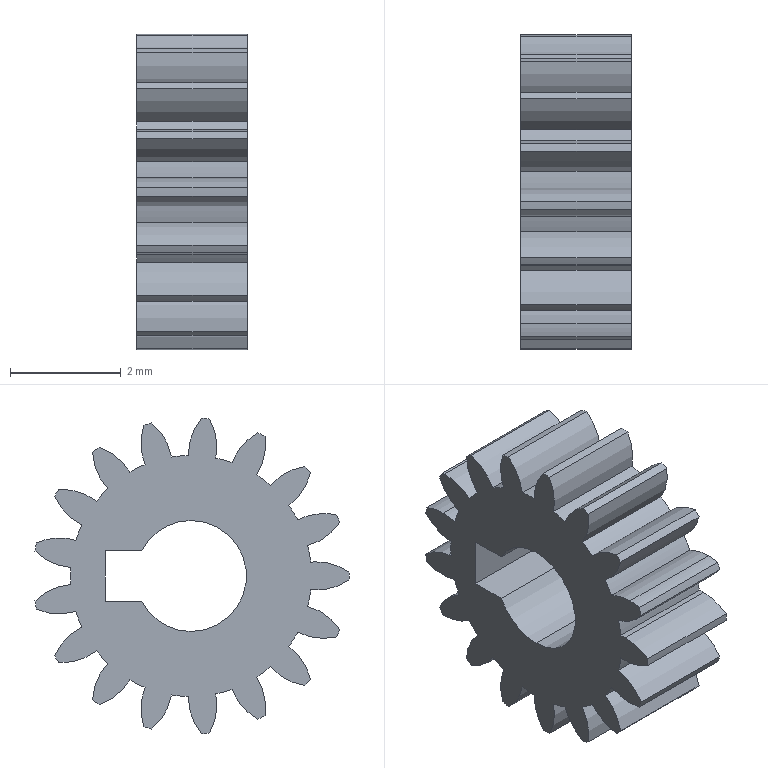Part | SolidWorks | features BaseBody 1, ICE 1 | 1 solid | 80 faces | box 2 x 5.664 x 5.687 mm | volume 31.821 mm3 | cylinder 75 | plane 5 | commonest cylinder face diameters 2.04 x38 4.348 x17 5.7 x17 2 x3